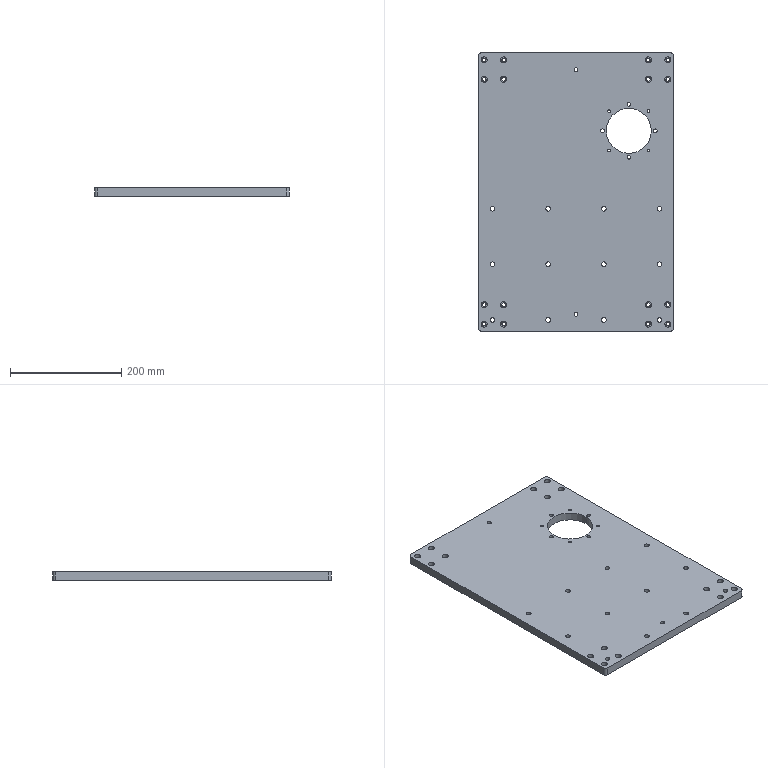Part | 1 solid | 148 faces | box 350 x 500 x 15 mm | volume 2516366 mm3 | cylinder 122 | plane 26 | commonest cylinder face diameters 6.6 x40 11 x40 8.5 x24 5 x8 6.8 x4 10 x4